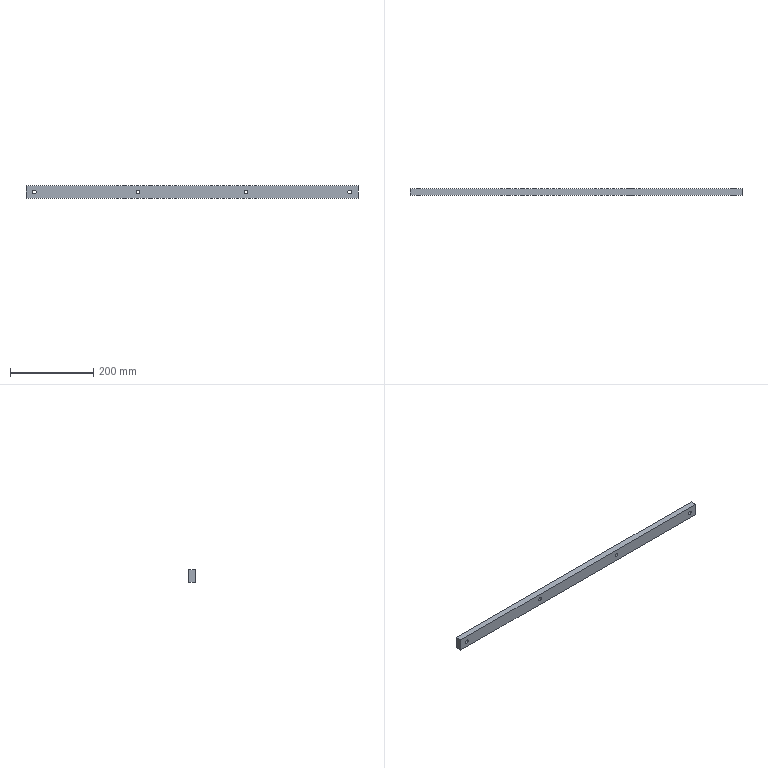Part | STEP file | 0244_210_Plate | 1 solid | 14 faces | box 800 x 15 x 30 mm | volume 356183 mm3 | cylinder 8 | plane 6 | commonest cylinder face diameters 9 x8
STEP:
#1=CARTESIAN_POINT('',(0.,0.,0.));
#2=DIRECTION('',(0.,0.,1.));
#3=DIRECTION('',(1.,0.,0.));
#4=AXIS2_PLACEMENT_3D('',#1,#2,#3);
#5=CARTESIAN_POINT('',(-130.,0.,19.5));
#6=VERTEX_POINT('',#5);
#7=CARTESIAN_POINT('',(-130.,15.,19.5));
#8=VERTEX_POINT('',#7);
#9=CARTESIAN_POINT('',(-130.,15.,19.5));
#10=DIRECTION('',(0.,1.,0.));
#11=VECTOR('',#10,1.);
#12=LINE('',#9,#11);
#13=CARTESIAN_POINT('',(-130.,15.,15.));
#14=DIRECTION('',(0.,1.,0.));
#15=DIRECTION('',(0.,0.,1.));
#16=AXIS2_PLACEMENT_3D('',#13,#14,#15);
#17=CYLINDRICAL_SURFACE('',#16,4.5);
#18=CARTESIAN_POINT('',(6.283,0.));
#19=DIRECTION('',(0.,1.));
#20=VECTOR('',#19,1.);
#21=LINE('',#18,#20);
#22=(GEOMETRIC_REPRESENTATION_CONTEXT(2)PARAMETRIC_REPRESENTATION_CONTEXT()REPRESENTATION_CONTEXT('',''));
#23=DEFINITIONAL_REPRESENTATION('',(#21),#22);
#24=PCURVE('',#17,#23);
#25=CARTESIAN_POINT('',(-130.,15.,15.));
#26=DIRECTION('',(0.,1.,0.));
#27=DIRECTION('',(0.,0.,1.));
#28=AXIS2_PLACEMENT_3D('',#25,#26,#27);
#29=CYLINDRICAL_SURFACE('',#28,4.5);
#30=CARTESIAN_POINT('',(0.,0.));
#31=DIRECTION('',(0.,1.));
#32=VECTOR('',#31,1.);
#33=LINE('',#30,#32);
#34=(GEOMETRIC_REPRESENTATION_CONTEXT(2)PARAMETRIC_REPRESENTATION_CONTEXT()REPRESENTATION_CONTEXT('',''));
#35=DEFINITIONAL_REPRESENTATION('',(#33),#34);
#36=PCURVE('',#29,#35);
#37=SURFACE_CURVE('',#12,(#24,#36),.PCURVE_S1.);
#38=EDGE_CURVE('',#6,#8,#37,.T.);
#39=ORIENTED_EDGE('',*,*,#38,.T.);
#40=CARTESIAN_POINT('',(-130.,15.,10.5));
#41=VERTEX_POINT('',#40);
#42=CARTESIAN_POINT('',(-130.,15.,15.));
#43=DIRECTION('',(0.,1.,0.));
#44=DIRECTION('',(0.,0.,1.));
#45=AXIS2_PLACEMENT_3D('',#42,#43,#44);
#46=CIRCLE('',#45,4.5);
#47=CARTESIAN_POINT('',(0.,0.));
#48=DIRECTION('',(1.,0.));
#49=VECTOR('',#48,1.);
#50=LINE('',#47,#49);
#51=(GEOMETRIC_REPRESENTATION_CONTEXT(2)PARAMETRIC_REPRESENTATION_CONTEXT()REPRESENTATION_CONTEXT('',''));
#52=DEFINITIONAL_REPRESENTATION('',(#50),#51);
#53=PCURVE('',#17,#52);
#54=CARTESIAN_POINT('',(-400.,15.,0.));
#55=DIRECTION('',(0.,1.,0.));
#56=DIRECTION('',(0.,0.,1.));
#57=AXIS2_PLACEMENT_3D('',#54,#55,#56);
#58=PLANE('',#57);
#59=CARTESIAN_POINT('',(15.,270.));
#60=DIRECTION('',(1.,0.));
#61=AXIS2_PLACEMENT_2D('',#59,#60);
#62=CIRCLE('',#61,4.5);
#63=(GEOMETRIC_REPRESENTATION_CONTEXT(2)PARAMETRIC_REPRESENTATION_CONTEXT()REPRESENTATION_CONTEXT('',''));
#64=DEFINITIONAL_REPRESENTATION('',(#62),#63);
#65=PCURVE('',#58,#64);
#66=SURFACE_CURVE('',#46,(#53,#65),.PCURVE_S1.);
#67=EDGE_CURVE('',#41,#8,#66,.T.);
#68=ORIENTED_EDGE('',*,*,#67,.F.);
#69=CARTESIAN_POINT('',(-130.,0.,10.5));
#70=VERTEX_POINT('',#69);
#71=CARTESIAN_POINT('',(-130.,15.,10.5));
#72=DIRECTION('',(0.,1.,0.));
#73=VECTOR('',#72,1.);
#74=LINE('',#71,#73);
#75=CARTESIAN_POINT('',(3.142,0.));
#76=DIRECTION('',(0.,1.));
#77=VECTOR('',#76,1.);
#78=LINE('',#75,#77);
#79=(GEOMETRIC_REPRESENTATION_CONTEXT(2)PARAMETRIC_REPRESENTATION_CONTEXT()REPRESENTATION_CONTEXT('',''));
#80=DEFINITIONAL_REPRESENTATION('',(#78),#79);
#81=PCURVE('',#17,#80);
#82=CARTESIAN_POINT('',(3.142,0.));
#83=DIRECTION('',(0.,1.));
#84=VECTOR('',#83,1.);
#85=LINE('',#82,#84);
#86=(GEOMETRIC_REPRESENTATION_CONTEXT(2)PARAMETRIC_REPRESENTATION_CONTEXT()REPRESENTATION_CONTEXT('',''));
#87=DEFINITIONAL_REPRESENTATION('',(#85),#86);
#88=PCURVE('',#29,#87);
#89=SURFACE_CURVE('',#74,(#81,#88),.PCURVE_S1.);
#90=EDGE_CURVE('',#70,#41,#89,.T.);
#91=ORIENTED_EDGE('',*,*,#90,.F.);
#92=CARTESIAN_POINT('',(-130.,0.,15.));
#93=DIRECTION('',(0.,1.,0.));
#94=DIRECTION('',(0.,0.,1.));
#95=AXIS2_PLACEMENT_3D('',#92,#93,#94);
#96=CIRCLE('',#95,4.5);
#97=CARTESIAN_POINT('',(0.,-15.));
#98=DIRECTION('',(1.,0.));
#99=VECTOR('',#98,1.);
#100=LINE('',#97,#99);
#101=(GEOMETRIC_REPRESENTATION_CONTEXT(2)PARAMETRIC_REPRESENTATION_CONTEXT()REPRESENTATION_CONTEXT('',''));
#102=DEFINITIONAL_REPRESENTATION('',(#100),#101);
#103=PCURVE('',#17,#102);
#104=CARTESIAN_POINT('',(-400.,0.,0.));
#105=DIRECTION('',(0.,1.,0.));
#106=DIRECTION('',(0.,0.,1.));
#107=AXIS2_PLACEMENT_3D('',#104,#105,#106);
#108=PLANE('',#107);
#109=CARTESIAN_POINT('',(15.,270.));
#110=DIRECTION('',(1.,0.));
#111=AXIS2_PLACEMENT_2D('',#109,#110);
#112=CIRCLE('',#111,4.5);
#113=(GEOMETRIC_REPRESENTATION_CONTEXT(2)PARAMETRIC_REPRESENTATION_CONTEXT()REPRESENTATION_CONTEXT('',''));
#114=DEFINITIONAL_REPRESENTATION('',(#112),#113);
#115=PCURVE('',#108,#114);
#116=SURFACE_CURVE('',#96,(#103,#115),.PCURVE_S1.);
#117=EDGE_CURVE('',#70,#6,#116,.T.);
#118=ORIENTED_EDGE('',*,*,#117,.T.);
#119=EDGE_LOOP('',(#39,#68,#91,#118));
#120=FACE_BOUND('',#119,.F.);
#121=ADVANCED_FACE('',(#120),#17,.F.);
#122=CARTESIAN_POINT('',(130.,0.,19.5));
#123=VERTEX_POINT('',#122);
#124=CARTESIAN_POINT('',(130.,15.,19.5));
#125=VERTEX_POINT('',#124);
#126=CARTESIAN_POINT('',(130.,15.,19.5));
#127=DIRECTION('',(0.,1.,0.));
#128=VECTOR('',#127,1.);
#129=LINE('',#126,#128);
#130=CARTESIAN_POINT('',(130.,15.,15.));
#131=DIRECTION('',(0.,1.,0.));
#132=DIRECTION('',(0.,0.,1.));
#133=AXIS2_PLACEMENT_3D('',#130,#131,#132);
#134=CYLINDRICAL_SURFACE('',#133,4.5);
#135=CARTESIAN_POINT('',(6.283,0.));
#136=DIRECTION('',(0.,1.));
#137=VECTOR('',#136,1.);
#138=LINE('',#135,#137);
#139=(GEOMETRIC_REPRESENTATION_CONTEXT(2)PARAMETRIC_REPRESENTATION_CONTEXT()REPRESENTATION_CONTEXT('',''));
#140=DEFINITIONAL_REPRESENTATION('',(#138),#139);
#141=PCURVE('',#134,#140);
#142=CARTESIAN_POINT('',(130.,15.,15.));
#143=DIRECTION('',(0.,1.,0.));
#144=DIRECTION('',(0.,0.,1.));
#145=AXIS2_PLACEMENT_3D('',#142,#143,#144);
#146=CYLINDRICAL_SURFACE('',#145,4.5);
#147=CARTESIAN_POINT('',(0.,0.));
#148=DIRECTION('',(0.,1.));
#149=VECTOR('',#148,1.);
#150=LINE('',#147,#149);
#151=(GEOMETRIC_REPRESENTATION_CONTEXT(2)PARAMETRIC_REPRESENTATION_CONTEXT()REPRESENTATION_CONTEXT('',''));
#152=DEFINITIONAL_REPRESENTATION('',(#150),#151);
#153=PCURVE('',#146,#152);
#154=SURFACE_CURVE('',#129,(#141,#153),.PCURVE_S1.);
#155=EDGE_CURVE('',#123,#125,#154,.T.);
#156=ORIENTED_EDGE('',*,*,#155,.T.);
#157=CARTESIAN_POINT('',(130.,15.,10.5));
#158=VERTEX_POINT('',#157);
#159=CARTESIAN_POINT('',(130.,15.,15.));
#160=DIRECTION('',(0.,1.,0.));
#161=DIRECTION('',(0.,0.,1.));
#162=AXIS2_PLACEMENT_3D('',#159,#160,#161);
#163=CIRCLE('',#162,4.5);
#164=CARTESIAN_POINT('',(0.,0.));
#165=DIRECTION('',(1.,0.));
#166=VECTOR('',#165,1.);
#167=LINE('',#164,#166);
#168=(GEOMETRIC_REPRESENTATION_CONTEXT(2)PARAMETRIC_REPRESENTATION_CONTEXT()REPRESENTATION_CONTEXT('',''));
#169=DEFINITIONAL_REPRESENTATION('',(#167),#168);
#170=PCURVE('',#134,#169);
#171=CARTESIAN_POINT('',(15.,530.));
#172=DIRECTION('',(1.,0.));
#173=AXIS2_PLACEMENT_2D('',#171,#172);
#174=CIRCLE('',#173,4.5);
#175=(GEOMETRIC_REPRESENTATION_CONTEXT(2)PARAMETRIC_REPRESENTATION_CONTEXT()REPRESENTATION_CONTEXT('',''));
#176=DEFINITIONAL_REPRESENTATION('',(#174),#175);
#177=PCURVE('',#58,#176);
#178=SURFACE_CURVE('',#163,(#170,#177),.PCURVE_S1.);
#179=EDGE_CURVE('',#158,#125,#178,.T.);
#180=ORIENTED_EDGE('',*,*,#179,.F.);
#181=CARTESIAN_POINT('',(130.,0.,10.5));
#182=VERTEX_POINT('',#181);
#183=CARTESIAN_POINT('',(130.,15.,10.5));
#184=DIRECTION('',(0.,1.,0.));
#185=VECTOR('',#184,1.);
#186=LINE('',#183,#185);
#187=CARTESIAN_POINT('',(3.142,0.));
#188=DIRECTION('',(0.,1.));
#189=VECTOR('',#188,1.);
#190=LINE('',#187,#189);
#191=(GEOMETRIC_REPRESENTATION_CONTEXT(2)PARAMETRIC_REPRESENTATION_CONTEXT()REPRESENTATION_CONTEXT('',''));
#192=DEFINITIONAL_REPRESENTATION('',(#190),#191);
#193=PCURVE('',#134,#192);
#194=CARTESIAN_POINT('',(3.142,0.));
#195=DIRECTION('',(0.,1.));
#196=VECTOR('',#195,1.);
#197=LINE('',#194,#196);
#198=(GEOMETRIC_REPRESENTATION_CONTEXT(2)PARAMETRIC_REPRESENTATION_CONTEXT()REPRESENTATION_CONTEXT('',''));
#199=DEFINITIONAL_REPRESENTATION('',(#197),#198);
#200=PCURVE('',#146,#199);
#201=SURFACE_CURVE('',#186,(#193,#200),.PCURVE_S1.);
#202=EDGE_CURVE('',#182,#158,#201,.T.);
#203=ORIENTED_EDGE('',*,*,#202,.F.);
#204=CARTESIAN_POINT('',(130.,0.,15.));
#205=DIRECTION('',(0.,1.,0.));
#206=DIRECTION('',(0.,0.,1.));
#207=AXIS2_PLACEMENT_3D('',#204,#205,#206);
#208=CIRCLE('',#207,4.5);
#209=CARTESIAN_POINT('',(0.,-15.));
#210=DIRECTION('',(1.,0.));
#211=VECTOR('',#210,1.);
#212=LINE('',#209,#211);
#213=(GEOMETRIC_REPRESENTATION_CONTEXT(2)PARAMETRIC_REPRESENTATION_CONTEXT()REPRESENTATION_CONTEXT('',''));
#214=DEFINITIONAL_REPRESENTATION('',(#212),#213);
#215=PCURVE('',#134,#214);
#216=CARTESIAN_POINT('',(15.,530.));
#217=DIRECTION('',(1.,0.));
#218=AXIS2_PLACEMENT_2D('',#216,#217);
#219=CIRCLE('',#218,4.5);
#220=(GEOMETRIC_REPRESENTATION_CONTEXT(2)PARAMETRIC_REPRESENTATION_CONTEXT()REPRESENTATION_CONTEXT('',''));
#221=DEFINITIONAL_REPRESENTATION('',(#219),#220);
#222=PCURVE('',#108,#221);
#223=SURFACE_CURVE('',#208,(#215,#222),.PCURVE_S1.);
#224=EDGE_CURVE('',#182,#123,#223,.T.);
#225=ORIENTED_EDGE('',*,*,#224,.T.);
#226=EDGE_LOOP('',(#156,#180,#203,#225));
#227=FACE_BOUND('',#226,.F.);
#228=ADVANCED_FACE('',(#227),#134,.F.);
#229=CARTESIAN_POINT('',(380.,0.,19.5));
#230=VERTEX_POINT('',#229);
#231=CARTESIAN_POINT('',(380.,15.,19.5));
#232=VERTEX_POINT('',#231);
#233=CARTESIAN_POINT('',(380.,15.,19.5));
#234=DIRECTION('',(0.,1.,0.));
#235=VECTOR('',#234,1.);
#236=LINE('',#233,#235);
#237=CARTESIAN_POINT('',(380.,15.,15.));
#238=DIRECTION('',(0.,1.,0.));
#239=DIRECTION('',(0.,0.,1.));
#240=AXIS2_PLACEMENT_3D('',#237,#238,#239);
#241=CYLINDRICAL_SURFACE('',#240,4.5);
#242=CARTESIAN_POINT('',(6.283,0.));
#243=DIRECTION('',(0.,1.));
#244=VECTOR('',#243,1.);
#245=LINE('',#242,#244);
#246=(GEOMETRIC_REPRESENTATION_CONTEXT(2)PARAMETRIC_REPRESENTATION_CONTEXT()REPRESENTATION_CONTEXT('',''));
#247=DEFINITIONAL_REPRESENTATION('',(#245),#246);
#248=PCURVE('',#241,#247);
#249=CARTESIAN_POINT('',(380.,15.,15.));
#250=DIRECTION('',(0.,1.,0.));
#251=DIRECTION('',(0.,0.,1.));
#252=AXIS2_PLACEMENT_3D('',#249,#250,#251);
#253=CYLINDRICAL_SURFACE('',#252,4.5);
#254=CARTESIAN_POINT('',(0.,0.));
#255=DIRECTION('',(0.,1.));
#256=VECTOR('',#255,1.);
#257=LINE('',#254,#256);
#258=(GEOMETRIC_REPRESENTATION_CONTEXT(2)PARAMETRIC_REPRESENTATION_CONTEXT()REPRESENTATION_CONTEXT('',''));
#259=DEFINITIONAL_REPRESENTATION('',(#257),#258);
#260=PCURVE('',#253,#259);
#261=SURFACE_CURVE('',#236,(#248,#260),.PCURVE_S1.);
#262=EDGE_CURVE('',#230,#232,#261,.T.);
#263=ORIENTED_EDGE('',*,*,#262,.T.);
#264=CARTESIAN_POINT('',(380.,15.,10.5));
#265=VERTEX_POINT('',#264);
#266=CARTESIAN_POINT('',(380.,15.,15.));
#267=DIRECTION('',(0.,1.,0.));
#268=DIRECTION('',(0.,0.,1.));
#269=AXIS2_PLACEMENT_3D('',#266,#267,#268);
#270=CIRCLE('',#269,4.5);
#271=CARTESIAN_POINT('',(0.,0.));
#272=DIRECTION('',(1.,0.));
#273=VECTOR('',#272,1.);
#274=LINE('',#271,#273);
#275=(GEOMETRIC_REPRESENTATION_CONTEXT(2)PARAMETRIC_REPRESENTATION_CONTEXT()REPRESENTATION_CONTEXT('',''));
#276=DEFINITIONAL_REPRESENTATION('',(#274),#275);
#277=PCURVE('',#241,#276);
#278=CARTESIAN_POINT('',(15.,780.));
#279=DIRECTION('',(1.,0.));
#280=AXIS2_PLACEMENT_2D('',#278,#279);
#281=CIRCLE('',#280,4.5);
#282=(GEOMETRIC_REPRESENTATION_CONTEXT(2)PARAMETRIC_REPRESENTATION_CONTEXT()REPRESENTATION_CONTEXT('',''));
#283=DEFINITIONAL_REPRESENTATION('',(#281),#282);
#284=PCURVE('',#58,#283);
#285=SURFACE_CURVE('',#270,(#277,#284),.PCURVE_S1.);
#286=EDGE_CURVE('',#265,#232,#285,.T.);
#287=ORIENTED_EDGE('',*,*,#286,.F.);
#288=CARTESIAN_POINT('',(380.,0.,10.5));
#289=VERTEX_POINT('',#288);
#290=CARTESIAN_POINT('',(380.,15.,10.5));
#291=DIRECTION('',(0.,1.,0.));
#292=VECTOR('',#291,1.);
#293=LINE('',#290,#292);
#294=CARTESIAN_POINT('',(3.142,0.));
#295=DIRECTION('',(0.,1.));
#296=VECTOR('',#295,1.);
#297=LINE('',#294,#296);
#298=(GEOMETRIC_REPRESENTATION_CONTEXT(2)PARAMETRIC_REPRESENTATION_CONTEXT()REPRESENTATION_CONTEXT('',''));
#299=DEFINITIONAL_REPRESENTATION('',(#297),#298);
#300=PCURVE('',#241,#299);
#301=CARTESIAN_POINT('',(3.142,0.));
#302=DIRECTION('',(0.,1.));
#303=VECTOR('',#302,1.);
#304=LINE('',#301,#303);
#305=(GEOMETRIC_REPRESENTATION_CONTEXT(2)PARAMETRIC_REPRESENTATION_CONTEXT()REPRESENTATION_CONTEXT('',''));
#306=DEFINITIONAL_REPRESENTATION('',(#304),#305);
#307=PCURVE('',#253,#306);
#308=SURFACE_CURVE('',#293,(#300,#307),.PCURVE_S1.);
#309=EDGE_CURVE('',#289,#265,#308,.T.);
#310=ORIENTED_EDGE('',*,*,#309,.F.);
#311=CARTESIAN_POINT('',(380.,0.,15.));
#312=DIRECTION('',(0.,1.,0.));
#313=DIRECTION('',(0.,0.,1.));
#314=AXIS2_PLACEMENT_3D('',#311,#312,#313);
#315=CIRCLE('',#314,4.5);
#316=CARTESIAN_POINT('',(0.,-15.));
#317=DIRECTION('',(1.,0.));
#318=VECTOR('',#317,1.);
#319=LINE('',#316,#318);
#320=(GEOMETRIC_REPRESENTATION_CONTEXT(2)PARAMETRIC_REPRESENTATION_CONTEXT()REPRESENTATION_CONTEXT('',''));
#321=DEFINITIONAL_REPRESENTATION('',(#319),#320);
#322=PCURVE('',#241,#321);
#323=CARTESIAN_POINT('',(15.,780.));
#324=DIRECTION('',(1.,0.));
#325=AXIS2_PLACEMENT_2D('',#323,#324);
#326=CIRCLE('',#325,4.5);
#327=(GEOMETRIC_REPRESENTATION_CONTEXT(2)PARAMETRIC_REPRESENTATION_CONTEXT()REPRESENTATION_CONTEXT('',''));
#328=DEFINITIONAL_REPRESENTATION('',(#326),#327);
#329=PCURVE('',#108,#328);
#330=SURFACE_CURVE('',#315,(#322,#329),.PCURVE_S1.);
#331=EDGE_CURVE('',#289,#230,#330,.T.);
#332=ORIENTED_EDGE('',*,*,#331,.T.);
#333=EDGE_LOOP('',(#263,#287,#310,#332));
#334=FACE_BOUND('',#333,.F.);
#335=ADVANCED_FACE('',(#334),#241,.F.);
#336=CARTESIAN_POINT('',(-380.,0.,19.5));
#337=VERTEX_POINT('',#336);
#338=CARTESIAN_POINT('',(-380.,15.,19.5));
#339=VERTEX_POINT('',#338);
#340=CARTESIAN_POINT('',(-380.,15.,19.5));
#341=DIRECTION('',(0.,1.,0.));
#342=VECTOR('',#341,1.);
#343=LINE('',#340,#342);
#344=CARTESIAN_POINT('',(-380.,15.,15.));
#345=DIRECTION('',(0.,1.,0.));
#346=DIRECTION('',(0.,0.,1.));
#347=AXIS2_PLACEMENT_3D('',#344,#345,#346);
#348=CYLINDRICAL_SURFACE('',#347,4.5);
#349=CARTESIAN_POINT('',(6.283,0.));
#350=DIRECTION('',(0.,1.));
#351=VECTOR('',#350,1.);
#352=LINE('',#349,#351);
#353=(GEOMETRIC_REPRESENTATION_CONTEXT(2)PARAMETRIC_REPRESENTATION_CONTEXT()REPRESENTATION_CONTEXT('',''));
#354=DEFINITIONAL_REPRESENTATION('',(#352),#353);
#355=PCURVE('',#348,#354);
#356=CARTESIAN_POINT('',(-380.,15.,15.));
#357=DIRECTION('',(0.,1.,0.));
#358=DIRECTION('',(0.,0.,1.));
#359=AXIS2_PLACEMENT_3D('',#356,#357,#358);
#360=CYLINDRICAL_SURFACE('',#359,4.5);
#361=CARTESIAN_POINT('',(0.,0.));
#362=DIRECTION('',(0.,1.));
#363=VECTOR('',#362,1.);
#364=LINE('',#361,#363);
#365=(GEOMETRIC_REPRESENTATION_CONTEXT(2)PARAMETRIC_REPRESENTATION_CONTEXT()REPRESENTATION_CONTEXT('',''));
#366=DEFINITIONAL_REPRESENTATION('',(#364),#365);
#367=PCURVE('',#360,#366);
#368=SURFACE_CURVE('',#343,(#355,#367),.PCURVE_S1.);
#369=EDGE_CURVE('',#337,#339,#368,.T.);
#370=ORIENTED_EDGE('',*,*,#369,.T.);
#371=CARTESIAN_POINT('',(-380.,15.,10.5));
#372=VERTEX_POINT('',#371);
#373=CARTESIAN_POINT('',(-380.,15.,15.));
#374=DIRECTION('',(0.,1.,0.));
#375=DIRECTION('',(0.,0.,1.));
#376=AXIS2_PLACEMENT_3D('',#373,#374,#375);
#377=CIRCLE('',#376,4.5);
#378=CARTESIAN_POINT('',(0.,0.));
#379=DIRECTION('',(1.,0.));
#380=VECTOR('',#379,1.);
#381=LINE('',#378,#380);
#382=(GEOMETRIC_REPRESENTATION_CONTEXT(2)PARAMETRIC_REPRESENTATION_CONTEXT()REPRESENTATION_CONTEXT('',''));
#383=DEFINITIONAL_REPRESENTATION('',(#381),#382);
#384=PCURVE('',#348,#383);
#385=CARTESIAN_POINT('',(15.,20.));
#386=DIRECTION('',(1.,0.));
#387=AXIS2_PLACEMENT_2D('',#385,#386);
#388=CIRCLE('',#387,4.5);
#389=(GEOMETRIC_REPRESENTATION_CONTEXT(2)PARAMETRIC_REPRESENTATION_CONTEXT()REPRESENTATION_CONTEXT('',''));
#390=DEFINITIONAL_REPRESENTATION('',(#388),#389);
#391=PCURVE('',#58,#390);
#392=SURFACE_CURVE('',#377,(#384,#391),.PCURVE_S1.);
#393=EDGE_CURVE('',#372,#339,#392,.T.);
#394=ORIENTED_EDGE('',*,*,#393,.F.);
#395=CARTESIAN_POINT('',(-380.,0.,10.5));
#396=VERTEX_POINT('',#395);
#397=CARTESIAN_POINT('',(-380.,15.,10.5));
#398=DIRECTION('',(0.,1.,0.));
#399=VECTOR('',#398,1.);
#400=LINE('',#397,#399);
#401=CARTESIAN_POINT('',(3.142,0.));
#402=DIRECTION('',(0.,1.));
#403=VECTOR('',#402,1.);
#404=LINE('',#401,#403);
#405=(GEOMETRIC_REPRESENTATION_CONTEXT(2)PARAMETRIC_REPRESENTATION_CONTEXT()REPRESENTATION_CONTEXT('',''));
#406=DEFINITIONAL_REPRESENTATION('',(#404),#405);
#407=PCURVE('',#348,#406);
#408=CARTESIAN_POINT('',(3.142,0.));
#409=DIRECTION('',(0.,1.));
#410=VECTOR('',#409,1.);
#411=LINE('',#408,#410);
#412=(GEOMETRIC_REPRESENTATION_CONTEXT(2)PARAMETRIC_REPRESENTATION_CONTEXT()REPRESENTATION_CONTEXT('',''));
#413=DEFINITIONAL_REPRESENTATION('',(#411),#412);
#414=PCURVE('',#360,#413);
#415=SURFACE_CURVE('',#400,(#407,#414),.PCURVE_S1.);
#416=EDGE_CURVE('',#396,#372,#415,.T.);
#417=ORIENTED_EDGE('',*,*,#416,.F.);
#418=CARTESIAN_POINT('',(-380.,0.,15.));
#419=DIRECTION('',(0.,1.,0.));
#420=DIRECTION('',(0.,0.,1.));
#421=AXIS2_PLACEMENT_3D('',#418,#419,#420);
#422=CIRCLE('',#421,4.5);
#423=CARTESIAN_POINT('',(0.,-15.));
#424=DIRECTION('',(1.,0.));
#425=VECTOR('',#424,1.);
#426=LINE('',#423,#425);
#427=(GEOMETRIC_REPRESENTATION_CONTEXT(2)PARAMETRIC_REPRESENTATION_CONTEXT()REPRESENTATION_CONTEXT('',''));
#428=DEFINITIONAL_REPRESENTATION('',(#426),#427);
#429=PCURVE('',#348,#428);
#430=CARTESIAN_POINT('',(15.,20.));
#431=DIRECTION('',(1.,0.));
#432=AXIS2_PLACEMENT_2D('',#430,#431);
#433=CIRCLE('',#432,4.5);
#434=(GEOMETRIC_REPRESENTATION_CONTEXT(2)PARAMETRIC_REPRESENTATION_CONTEXT()REPRESENTATION_CONTEXT('',''));
#435=DEFINITIONAL_REPRESENTATION('',(#433),#434);
#436=PCURVE('',#108,#435);
#437=SURFACE_CURVE('',#422,(#429,#436),.PCURVE_S1.);
#438=EDGE_CURVE('',#396,#337,#437,.T.);
#439=ORIENTED_EDGE('',*,*,#438,.T.);
#440=EDGE_LOOP('',(#370,#394,#417,#439));
#441=FACE_BOUND('',#440,.F.);
#442=ADVANCED_FACE('',(#441),#348,.F.);
#443=CARTESIAN_POINT('',(400.,0.,0.));
#444=VERTEX_POINT('',#443);
#445=CARTESIAN_POINT('',(-400.,0.,0.));
#446=VERTEX_POINT('',#445);
#447=CARTESIAN_POINT('',(400.,0.,0.));
#448=DIRECTION('',(-1.,0.,0.));
#449=VECTOR('',#448,1.);
#450=LINE('',#447,#449);
#451=CARTESIAN_POINT('',(400.,15.,0.));
#452=DIRECTION('',(0.,0.,1.));
#453=DIRECTION('',(1.,0.,0.));
#454=AXIS2_PLACEMENT_3D('',#451,#452,#453);
#455=PLANE('',#454);
#456=CARTESIAN_POINT('',(0.,-15.));
#457=DIRECTION('',(-1.,0.));
#458=VECTOR('',#457,1.);
#459=LINE('',#456,#458);
#460=(GEOMETRIC_REPRESENTATION_CONTEXT(2)PARAMETRIC_REPRESENTATION_CONTEXT()REPRESENTATION_CONTEXT('',''));
#461=DEFINITIONAL_REPRESENTATION('',(#459),#460);
#462=PCURVE('',#455,#461);
#463=CARTESIAN_POINT('',(0.,800.));
#464=DIRECTION('',(0.,-1.));
#465=VECTOR('',#464,1.);
#466=LINE('',#463,#465);
#467=(GEOMETRIC_REPRESENTATION_CONTEXT(2)PARAMETRIC_REPRESENTATION_CONTEXT()REPRESENTATION_CONTEXT('',''));
#468=DEFINITIONAL_REPRESENTATION('',(#466),#467);
#469=PCURVE('',#108,#468);
#470=SURFACE_CURVE('',#450,(#462,#469),.PCURVE_S1.);
#471=EDGE_CURVE('',#444,#446,#470,.T.);
#472=ORIENTED_EDGE('',*,*,#471,.T.);
#473=CARTESIAN_POINT('',(-400.,15.,0.));
#474=VERTEX_POINT('',#473);
#475=CARTESIAN_POINT('',(-400.,15.,0.));
#476=DIRECTION('',(0.,-1.,0.));
#477=VECTOR('',#476,1.);
#478=LINE('',#475,#477);
#479=CARTESIAN_POINT('',(-800.,0.));
#480=DIRECTION('',(0.,-1.));
#481=VECTOR('',#480,1.);
#482=LINE('',#479,#481);
#483=(GEOMETRIC_REPRESENTATION_CONTEXT(2)PARAMETRIC_REPRESENTATION_CONTEXT()REPRESENTATION_CONTEXT('',''));
#484=DEFINITIONAL_REPRESENTATION('',(#482),#483);
#485=PCURVE('',#455,#484);
#486=CARTESIAN_POINT('',(-400.,15.,0.));
#487=DIRECTION('',(1.,0.,0.));
#488=DIRECTION('',(0.,0.,-1.));
#489=AXIS2_PLACEMENT_3D('',#486,#487,#488);
#490=PLANE('',#489);
#491=CARTESIAN_POINT('',(0.,0.));
#492=DIRECTION('',(0.,-1.));
#493=VECTOR('',#492,1.);
#494=LINE('',#491,#493);
#495=(GEOMETRIC_REPRESENTATION_CONTEXT(2)PARAMETRIC_REPRESENTATION_CONTEXT()REPRESENTATION_CONTEXT('',''));
#496=DEFINITIONAL_REPRESENTATION('',(#494),#495);
#497=PCURVE('',#490,#496);
#498=SURFACE_CURVE('',#478,(#485,#497),.PCURVE_S1.);
#499=EDGE_CURVE('',#474,#446,#498,.T.);
#500=ORIENTED_EDGE('',*,*,#499,.F.);
#501=CARTESIAN_POINT('',(400.,15.,0.));
#502=VERTEX_POINT('',#501);
#503=CARTESIAN_POINT('',(400.,15.,0.));
#504=DIRECTION('',(-1.,0.,0.));
#505=VECTOR('',#504,1.);
#506=LINE('',#503,#505);
#507=CARTESIAN_POINT('',(0.,0.));
#508=DIRECTION('',(-1.,0.));
#509=VECTOR('',#508,1.);
#510=LINE('',#507,#509);
#511=(GEOMETRIC_REPRESENTATION_CONTEXT(2)PARAMETRIC_REPRESENTATION_CONTEXT()REPRESENTATION_CONTEXT('',''));
#512=DEFINITIONAL_REPRESENTATION('',(#510),#511);
#513=PCURVE('',#455,#512);
#514=CARTESIAN_POINT('',(0.,800.));
#515=DIRECTION('',(0.,-1.));
#516=VECTOR('',#515,1.);
#517=LINE('',#514,#516);
#518=(GEOMETRIC_REPRESENTATION_CONTEXT(2)PARAMETRIC_REPRESENTATION_CONTEXT()REPRESENTATION_CONTEXT('',''));
#519=DEFINITIONAL_REPRESENTATION('',(#517),#518);
#520=PCURVE('',#58,#519);
#521=SURFACE_CURVE('',#506,(#513,#520),.PCURVE_S1.);
#522=EDGE_CURVE('',#502,#474,#521,.T.);
#523=ORIENTED_EDGE('',*,*,#522,.F.);
#524=CARTESIAN_POINT('',(400.,15.,0.));
#525=DIRECTION('',(0.,-1.,0.));
#526=VECTOR('',#525,1.);
#527=LINE('',#524,#526);
#528=CARTESIAN_POINT('',(0.,0.));
#529=DIRECTION('',(0.,-1.));
#530=VECTOR('',#529,1.);
#531=LINE('',#528,#530);
#532=(GEOMETRIC_REPRESENTATION_CONTEXT(2)PARAMETRIC_REPRESENTATION_CONTEXT()REPRESENTATION_CONTEXT('',''));
#533=DEFINITIONAL_REPRESENTATION('',(#531),#532);
#534=PCURVE('',#455,#533);
#535=CARTESIAN_POINT('',(400.,15.,0.));
#536=DIRECTION('',(-1.,0.,0.));
#537=DIRECTION('',(0.,0.,1.));
#538=AXIS2_PLACEMENT_3D('',#535,#536,#537);
#539=PLANE('',#538);
#540=CARTESIAN_POINT('',(0.,0.));
#541=DIRECTION('',(0.,-1.));
#542=VECTOR('',#541,1.);
#543=LINE('',#540,#542);
#544=(GEOMETRIC_REPRESENTATION_CONTEXT(2)PARAMETRIC_REPRESENTATION_CONTEXT()REPRESENTATION_CONTEXT('',''));
#545=DEFINITIONAL_REPRESENTATION('',(#543),#544);
#546=PCURVE('',#539,#545);
#547=SURFACE_CURVE('',#527,(#534,#546),.PCURVE_S1.);
#548=EDGE_CURVE('',#502,#444,#547,.T.);
#549=ORIENTED_EDGE('',*,*,#548,.T.);
#550=EDGE_LOOP('',(#472,#500,#523,#549));
#551=FACE_BOUND('',#550,.T.);
#552=ADVANCED_FACE('',(#551),#455,.F.);
#553=CARTESIAN_POINT('',(-400.,0.,30.));
#554=VERTEX_POINT('',#553);
#555=CARTESIAN_POINT('',(-400.,0.,0.));
#556=DIRECTION('',(0.,0.,1.));
#557=VECTOR('',#556,1.);
#558=LINE('',#555,#557);
#559=CARTESIAN_POINT('',(0.,-15.));
#560=DIRECTION('',(-1.,0.));
#561=VECTOR('',#560,1.);
#562=LINE('',#559,#561);
#563=(GEOMETRIC_REPRESENTATION_CONTEXT(2)PARAMETRIC_REPRESENTATION_CONTEXT()REPRESENTATION_CONTEXT('',''));
#564=DEFINITIONAL_REPRESENTATION('',(#562),#563);
#565=PCURVE('',#490,#564);
#566=CARTESIAN_POINT('',(0.,0.));
#567=DIRECTION('',(1.,0.));
#568=VECTOR('',#567,1.);
#569=LINE('',#566,#568);
#570=(GEOMETRIC_REPRESENTATION_CONTEXT(2)PARAMETRIC_REPRESENTATION_CONTEXT()REPRESENTATION_CONTEXT('',''));
#571=DEFINITIONAL_REPRESENTATION('',(#569),#570);
#572=PCURVE('',#108,#571);
#573=SURFACE_CURVE('',#558,(#565,#572),.PCURVE_S1.);
#574=EDGE_CURVE('',#446,#554,#573,.T.);
#575=ORIENTED_EDGE('',*,*,#574,.T.);
#576=CARTESIAN_POINT('',(-400.,15.,30.));
#577=VERTEX_POINT('',#576);
#578=CARTESIAN_POINT('',(-400.,15.,30.));
#579=DIRECTION('',(0.,-1.,0.));
#580=VECTOR('',#579,1.);
#581=LINE('',#578,#580);
#582=CARTESIAN_POINT('',(-30.,0.));
#583=DIRECTION('',(0.,-1.));
#584=VECTOR('',#583,1.);
#585=LINE('',#582,#584);
#586=(GEOMETRIC_REPRESENTATION_CONTEXT(2)PARAMETRIC_REPRESENTATION_CONTEXT()REPRESENTATION_CONTEXT('',''));
#587=DEFINITIONAL_REPRESENTATION('',(#585),#586);
#588=PCURVE('',#490,#587);
#589=CARTESIAN_POINT('',(400.,15.,30.));
#590=DIRECTION('',(0.,0.,-1.));
#591=DIRECTION('',(-1.,0.,0.));
#592=AXIS2_PLACEMENT_3D('',#589,#590,#591);
#593=PLANE('',#592);
#594=CARTESIAN_POINT('',(800.,0.));
#595=DIRECTION('',(0.,-1.));
#596=VECTOR('',#595,1.);
#597=LINE('',#594,#596);
#598=(GEOMETRIC_REPRESENTATION_CONTEXT(2)PARAMETRIC_REPRESENTATION_CONTEXT()REPRESENTATION_CONTEXT('',''));
#599=DEFINITIONAL_REPRESENTATION('',(#597),#598);
#600=PCURVE('',#593,#599);
#601=SURFACE_CURVE('',#581,(#588,#600),.PCURVE_S1.);
#602=EDGE_CURVE('',#577,#554,#601,.T.);
#603=ORIENTED_EDGE('',*,*,#602,.F.);
#604=CARTESIAN_POINT('',(-400.,15.,0.));
#605=DIRECTION('',(0.,0.,1.));
#606=VECTOR('',#605,1.);
#607=LINE('',#604,#606);
#608=CARTESIAN_POINT('',(0.,0.));
#609=DIRECTION('',(-1.,0.));
#610=VECTOR('',#609,1.);
#611=LINE('',#608,#610);
#612=(GEOMETRIC_REPRESENTATION_CONTEXT(2)PARAMETRIC_REPRESENTATION_CONTEXT()REPRESENTATION_CONTEXT('',''));
#613=DEFINITIONAL_REPRESENTATION('',(#611),#612);
#614=PCURVE('',#490,#613);
#615=CARTESIAN_POINT('',(0.,0.));
#616=DIRECTION('',(1.,0.));
#617=VECTOR('',#616,1.);
#618=LINE('',#615,#617);
#619=(GEOMETRIC_REPRESENTATION_CONTEXT(2)PARAMETRIC_REPRESENTATION_CONTEXT()REPRESENTATION_CONTEXT('',''));
#620=DEFINITIONAL_REPRESENTATION('',(#618),#619);
#621=PCURVE('',#58,#620);
#622=SURFACE_CURVE('',#607,(#614,#621),.PCURVE_S1.);
#623=EDGE_CURVE('',#474,#577,#622,.T.);
#624=ORIENTED_EDGE('',*,*,#623,.F.);
#625=ORIENTED_EDGE('',*,*,#499,.T.);
#626=EDGE_LOOP('',(#575,#603,#624,#625));
#627=FACE_BOUND('',#626,.T.);
#628=ADVANCED_FACE('',(#627),#490,.F.);
#629=CARTESIAN_POINT('',(400.,0.,30.));
#630=VERTEX_POINT('',#629);
#631=CARTESIAN_POINT('',(400.,0.,30.));
#632=DIRECTION('',(1.,0.,0.));
#633=VECTOR('',#632,1.);
#634=LINE('',#631,#633);
#635=CARTESIAN_POINT('',(0.,-15.));
#636=DIRECTION('',(-1.,0.));
#637=VECTOR('',#636,1.);
#638=LINE('',#635,#637);
#639=(GEOMETRIC_REPRESENTATION_CONTEXT(2)PARAMETRIC_REPRESENTATION_CONTEXT()REPRESENTATION_CONTEXT('',''));
#640=DEFINITIONAL_REPRESENTATION('',(#638),#639);
#641=PCURVE('',#593,#640);
#642=CARTESIAN_POINT('',(30.,800.));
#643=DIRECTION('',(0.,1.));
#644=VECTOR('',#643,1.);
#645=LINE('',#642,#644);
#646=(GEOMETRIC_REPRESENTATION_CONTEXT(2)PARAMETRIC_REPRESENTATION_CONTEXT()REPRESENTATION_CONTEXT('',''));
#647=DEFINITIONAL_REPRESENTATION('',(#645),#646);
#648=PCURVE('',#108,#647);
#649=SURFACE_CURVE('',#634,(#641,#648),.PCURVE_S1.);
#650=EDGE_CURVE('',#554,#630,#649,.T.);
#651=ORIENTED_EDGE('',*,*,#650,.T.);
#652=CARTESIAN_POINT('',(400.,15.,30.));
#653=VERTEX_POINT('',#652);
#654=CARTESIAN_POINT('',(400.,15.,30.));
#655=DIRECTION('',(0.,-1.,0.));
#656=VECTOR('',#655,1.);
#657=LINE('',#654,#656);
#658=CARTESIAN_POINT('',(0.,0.));
#659=DIRECTION('',(0.,-1.));
#660=VECTOR('',#659,1.);
#661=LINE('',#658,#660);
#662=(GEOMETRIC_REPRESENTATION_CONTEXT(2)PARAMETRIC_REPRESENTATION_CONTEXT()REPRESENTATION_CONTEXT('',''));
#663=DEFINITIONAL_REPRESENTATION('',(#661),#662);
#664=PCURVE('',#593,#663);
#665=CARTESIAN_POINT('',(30.,0.));
#666=DIRECTION('',(0.,-1.));
#667=VECTOR('',#666,1.);
#668=LINE('',#665,#667);
#669=(GEOMETRIC_REPRESENTATION_CONTEXT(2)PARAMETRIC_REPRESENTATION_CONTEXT()REPRESENTATION_CONTEXT('',''));
#670=DEFINITIONAL_REPRESENTATION('',(#668),#669);
#671=PCURVE('',#539,#670);
#672=SURFACE_CURVE('',#657,(#664,#671),.PCURVE_S1.);
#673=EDGE_CURVE('',#653,#630,#672,.T.);
#674=ORIENTED_EDGE('',*,*,#673,.F.);
#675=CARTESIAN_POINT('',(400.,15.,30.));
#676=DIRECTION('',(1.,0.,0.));
#677=VECTOR('',#676,1.);
#678=LINE('',#675,#677);
#679=CARTESIAN_POINT('',(0.,0.));
#680=DIRECTION('',(-1.,0.));
#681=VECTOR('',#680,1.);
#682=LINE('',#679,#681);
#683=(GEOMETRIC_REPRESENTATION_CONTEXT(2)PARAMETRIC_REPRESENTATION_CONTEXT()REPRESENTATION_CONTEXT('',''));
#684=DEFINITIONAL_REPRESENTATION('',(#682),#683);
#685=PCURVE('',#593,#684);
#686=CARTESIAN_POINT('',(30.,800.));
#687=DIRECTION('',(0.,1.));
#688=VECTOR('',#687,1.);
#689=LINE('',#686,#688);
#690=(GEOMETRIC_REPRESENTATION_CONTEXT(2)PARAMETRIC_REPRESENTATION_CONTEXT()REPRESENTATION_CONTEXT('',''));
#691=DEFINITIONAL_REPRESENTATION('',(#689),#690);
#692=PCURVE('',#58,#691);
#693=SURFACE_CURVE('',#678,(#685,#692),.PCURVE_S1.);
#694=EDGE_CURVE('',#577,#653,#693,.T.);
#695=ORIENTED_EDGE('',*,*,#694,.F.);
#696=ORIENTED_EDGE('',*,*,#602,.T.);
#697=EDGE_LOOP('',(#651,#674,#695,#696));
#698=FACE_BOUND('',#697,.T.);
#699=ADVANCED_FACE('',(#698),#593,.F.);
#700=CARTESIAN_POINT('',(400.,0.,0.));
#701=DIRECTION('',(0.,0.,-1.));
#702=VECTOR('',#701,1.);
#703=LINE('',#700,#702);
#704=CARTESIAN_POINT('',(0.,-15.));
#705=DIRECTION('',(-1.,0.));
#706=VECTOR('',#705,1.);
#707=LINE('',#704,#706);
#708=(GEOMETRIC_REPRESENTATION_CONTEXT(2)PARAMETRIC_REPRESENTATION_CONTEXT()REPRESENTATION_CONTEXT('',''));
#709=DEFINITIONAL_REPRESENTATION('',(#707),#708);
#710=PCURVE('',#539,#709);
#711=CARTESIAN_POINT('',(0.,800.));
#712=DIRECTION('',(-1.,0.));
#713=VECTOR('',#712,1.);
#714=LINE('',#711,#713);
#715=(GEOMETRIC_REPRESENTATION_CONTEXT(2)PARAMETRIC_REPRESENTATION_CONTEXT()REPRESENTATION_CONTEXT('',''));
#716=DEFINITIONAL_REPRESENTATION('',(#714),#715);
#717=PCURVE('',#108,#716);
#718=SURFACE_CURVE('',#703,(#710,#717),.PCURVE_S1.);
#719=EDGE_CURVE('',#630,#444,#718,.T.);
#720=ORIENTED_EDGE('',*,*,#719,.T.);
#721=ORIENTED_EDGE('',*,*,#548,.F.);
#722=CARTESIAN_POINT('',(400.,15.,0.));
#723=DIRECTION('',(0.,0.,-1.));
#724=VECTOR('',#723,1.);
#725=LINE('',#722,#724);
#726=CARTESIAN_POINT('',(0.,0.));
#727=DIRECTION('',(-1.,0.));
#728=VECTOR('',#727,1.);
#729=LINE('',#726,#728);
#730=(GEOMETRIC_REPRESENTATION_CONTEXT(2)PARAMETRIC_REPRESENTATION_CONTEXT()REPRESENTATION_CONTEXT('',''));
#731=DEFINITIONAL_REPRESENTATION('',(#729),#730);
#732=PCURVE('',#539,#731);
#733=CARTESIAN_POINT('',(0.,800.));
#734=DIRECTION('',(-1.,0.));
#735=VECTOR('',#734,1.);
#736=LINE('',#733,#735);
#737=(GEOMETRIC_REPRESENTATION_CONTEXT(2)PARAMETRIC_REPRESENTATION_CONTEXT()REPRESENTATION_CONTEXT('',''));
#738=DEFINITIONAL_REPRESENTATION('',(#736),#737);
#739=PCURVE('',#58,#738);
#740=SURFACE_CURVE('',#725,(#732,#739),.PCURVE_S1.);
#741=EDGE_CURVE('',#653,#502,#740,.T.);
#742=ORIENTED_EDGE('',*,*,#741,.F.);
#743=ORIENTED_EDGE('',*,*,#673,.T.);
#744=EDGE_LOOP('',(#720,#721,#742,#743));
#745=FACE_BOUND('',#744,.T.);
#746=ADVANCED_FACE('',(#745),#539,.F.);
#747=CARTESIAN_POINT('',(-130.,15.,15.));
#748=DIRECTION('',(0.,1.,0.));
#749=DIRECTION('',(0.,0.,1.));
#750=AXIS2_PLACEMENT_3D('',#747,#748,#749);
#751=CIRCLE('',#750,4.5);
#752=CARTESIAN_POINT('',(15.,270.));
#753=DIRECTION('',(1.,0.));
#754=AXIS2_PLACEMENT_2D('',#752,#753);
#755=CIRCLE('',#754,4.5);
#756=(GEOMETRIC_REPRESENTATION_CONTEXT(2)PARAMETRIC_REPRESENTATION_CONTEXT()REPRESENTATION_CONTEXT('',''));
#757=DEFINITIONAL_REPRESENTATION('',(#755),#756);
#758=PCURVE('',#58,#757);
#759=CARTESIAN_POINT('',(0.,0.));
#760=DIRECTION('',(1.,0.));
#761=VECTOR('',#760,1.);
#762=LINE('',#759,#761);
#763=(GEOMETRIC_REPRESENTATION_CONTEXT(2)PARAMETRIC_REPRESENTATION_CONTEXT()REPRESENTATION_CONTEXT('',''));
#764=DEFINITIONAL_REPRESENTATION('',(#762),#763);
#765=PCURVE('',#29,#764);
#766=SURFACE_CURVE('',#751,(#758,#765),.PCURVE_S1.);
#767=EDGE_CURVE('',#8,#41,#766,.T.);
#768=ORIENTED_EDGE('',*,*,#767,.F.);
#769=ORIENTED_EDGE('',*,*,#67,.F.);
#770=EDGE_LOOP('',(#768,#769));
#771=FACE_BOUND('',#770,.T.);
#772=CARTESIAN_POINT('',(130.,15.,15.));
#773=DIRECTION('',(0.,1.,0.));
#774=DIRECTION('',(0.,0.,1.));
#775=AXIS2_PLACEMENT_3D('',#772,#773,#774);
#776=CIRCLE('',#775,4.5);
#777=CARTESIAN_POINT('',(15.,530.));
#778=DIRECTION('',(1.,0.));
#779=AXIS2_PLACEMENT_2D('',#777,#778);
#780=CIRCLE('',#779,4.5);
#781=(GEOMETRIC_REPRESENTATION_CONTEXT(2)PARAMETRIC_REPRESENTATION_CONTEXT()REPRESENTATION_CONTEXT('',''));
#782=DEFINITIONAL_REPRESENTATION('',(#780),#781);
#783=PCURVE('',#58,#782);
#784=CARTESIAN_POINT('',(0.,0.));
#785=DIRECTION('',(1.,0.));
#786=VECTOR('',#785,1.);
#787=LINE('',#784,#786);
#788=(GEOMETRIC_REPRESENTATION_CONTEXT(2)PARAMETRIC_REPRESENTATION_CONTEXT()REPRESENTATION_CONTEXT('',''));
#789=DEFINITIONAL_REPRESENTATION('',(#787),#788);
#790=PCURVE('',#146,#789);
#791=SURFACE_CURVE('',#776,(#783,#790),.PCURVE_S1.);
#792=EDGE_CURVE('',#125,#158,#791,.T.);
#793=ORIENTED_EDGE('',*,*,#792,.F.);
#794=ORIENTED_EDGE('',*,*,#179,.F.);
#795=EDGE_LOOP('',(#793,#794));
#796=FACE_BOUND('',#795,.T.);
#797=CARTESIAN_POINT('',(380.,15.,15.));
#798=DIRECTION('',(0.,1.,0.));
#799=DIRECTION('',(0.,0.,1.));
#800=AXIS2_PLACEMENT_3D('',#797,#798,#799);
#801=CIRCLE('',#800,4.5);
#802=CARTESIAN_POINT('',(15.,780.));
#803=DIRECTION('',(1.,0.));
#804=AXIS2_PLACEMENT_2D('',#802,#803);
#805=CIRCLE('',#804,4.5);
#806=(GEOMETRIC_REPRESENTATION_CONTEXT(2)PARAMETRIC_REPRESENTATION_CONTEXT()REPRESENTATION_CONTEXT('',''));
#807=DEFINITIONAL_REPRESENTATION('',(#805),#806);
#808=PCURVE('',#58,#807);
#809=CARTESIAN_POINT('',(0.,0.));
#810=DIRECTION('',(1.,0.));
#811=VECTOR('',#810,1.);
#812=LINE('',#809,#811);
#813=(GEOMETRIC_REPRESENTATION_CONTEXT(2)PARAMETRIC_REPRESENTATION_CONTEXT()REPRESENTATION_CONTEXT('',''));
#814=DEFINITIONAL_REPRESENTATION('',(#812),#813);
#815=PCURVE('',#253,#814);
#816=SURFACE_CURVE('',#801,(#808,#815),.PCURVE_S1.);
#817=EDGE_CURVE('',#232,#265,#816,.T.);
#818=ORIENTED_EDGE('',*,*,#817,.F.);
#819=ORIENTED_EDGE('',*,*,#286,.F.);
#820=EDGE_LOOP('',(#818,#819));
#821=FACE_BOUND('',#820,.T.);
#822=CARTESIAN_POINT('',(-380.,15.,15.));
#823=DIRECTION('',(0.,1.,0.));
#824=DIRECTION('',(0.,0.,1.));
#825=AXIS2_PLACEMENT_3D('',#822,#823,#824);
#826=CIRCLE('',#825,4.5);
#827=CARTESIAN_POINT('',(15.,20.));
#828=DIRECTION('',(1.,0.));
#829=AXIS2_PLACEMENT_2D('',#827,#828);
#830=CIRCLE('',#829,4.5);
#831=(GEOMETRIC_REPRESENTATION_CONTEXT(2)PARAMETRIC_REPRESENTATION_CONTEXT()REPRESENTATION_CONTEXT('',''));
#832=DEFINITIONAL_REPRESENTATION('',(#830),#831);
#833=PCURVE('',#58,#832);
#834=CARTESIAN_POINT('',(0.,0.));
#835=DIRECTION('',(1.,0.));
#836=VECTOR('',#835,1.);
#837=LINE('',#834,#836);
#838=(GEOMETRIC_REPRESENTATION_CONTEXT(2)PARAMETRIC_REPRESENTATION_CONTEXT()REPRESENTATION_CONTEXT('',''));
#839=DEFINITIONAL_REPRESENTATION('',(#837),#838);
#840=PCURVE('',#360,#839);
#841=SURFACE_CURVE('',#826,(#833,#840),.PCURVE_S1.);
#842=EDGE_CURVE('',#339,#372,#841,.T.);
#843=ORIENTED_EDGE('',*,*,#842,.F.);
#844=ORIENTED_EDGE('',*,*,#393,.F.);
#845=EDGE_LOOP('',(#843,#844));
#846=FACE_BOUND('',#845,.T.);
#847=ORIENTED_EDGE('',*,*,#522,.T.);
#848=ORIENTED_EDGE('',*,*,#623,.T.);
#849=ORIENTED_EDGE('',*,*,#694,.T.);
#850=ORIENTED_EDGE('',*,*,#741,.T.);
#851=EDGE_LOOP('',(#847,#848,#849,#850));
#852=FACE_BOUND('',#851,.T.);
#853=ADVANCED_FACE('',(#771,#796,#821,#846,#852),#58,.T.);
#854=CARTESIAN_POINT('',(-130.,0.,15.));
#855=DIRECTION('',(0.,1.,0.));
#856=DIRECTION('',(0.,0.,1.));
#857=AXIS2_PLACEMENT_3D('',#854,#855,#856);
#858=CIRCLE('',#857,4.5);
#859=CARTESIAN_POINT('',(15.,270.));
#860=DIRECTION('',(1.,0.));
#861=AXIS2_PLACEMENT_2D('',#859,#860);
#862=CIRCLE('',#861,4.5);
#863=(GEOMETRIC_REPRESENTATION_CONTEXT(2)PARAMETRIC_REPRESENTATION_CONTEXT()REPRESENTATION_CONTEXT('',''));
#864=DEFINITIONAL_REPRESENTATION('',(#862),#863);
#865=PCURVE('',#108,#864);
#866=CARTESIAN_POINT('',(0.,-15.));
#867=DIRECTION('',(1.,0.));
#868=VECTOR('',#867,1.);
#869=LINE('',#866,#868);
#870=(GEOMETRIC_REPRESENTATION_CONTEXT(2)PARAMETRIC_REPRESENTATION_CONTEXT()REPRESENTATION_CONTEXT('',''));
#871=DEFINITIONAL_REPRESENTATION('',(#869),#870);
#872=PCURVE('',#29,#871);
#873=SURFACE_CURVE('',#858,(#865,#872),.PCURVE_S1.);
#874=EDGE_CURVE('',#6,#70,#873,.T.);
#875=ORIENTED_EDGE('',*,*,#874,.T.);
#876=ORIENTED_EDGE('',*,*,#117,.T.);
#877=EDGE_LOOP('',(#875,#876));
#878=FACE_BOUND('',#877,.T.);
#879=CARTESIAN_POINT('',(130.,0.,15.));
#880=DIRECTION('',(0.,1.,0.));
#881=DIRECTION('',(0.,0.,1.));
#882=AXIS2_PLACEMENT_3D('',#879,#880,#881);
#883=CIRCLE('',#882,4.5);
#884=CARTESIAN_POINT('',(15.,530.));
#885=DIRECTION('',(1.,0.));
#886=AXIS2_PLACEMENT_2D('',#884,#885);
#887=CIRCLE('',#886,4.5);
#888=(GEOMETRIC_REPRESENTATION_CONTEXT(2)PARAMETRIC_REPRESENTATION_CONTEXT()REPRESENTATION_CONTEXT('',''));
#889=DEFINITIONAL_REPRESENTATION('',(#887),#888);
#890=PCURVE('',#108,#889);
#891=CARTESIAN_POINT('',(0.,-15.));
#892=DIRECTION('',(1.,0.));
#893=VECTOR('',#892,1.);
#894=LINE('',#891,#893);
#895=(GEOMETRIC_REPRESENTATION_CONTEXT(2)PARAMETRIC_REPRESENTATION_CONTEXT()REPRESENTATION_CONTEXT('',''));
#896=DEFINITIONAL_REPRESENTATION('',(#894),#895);
#897=PCURVE('',#146,#896);
#898=SURFACE_CURVE('',#883,(#890,#897),.PCURVE_S1.);
#899=EDGE_CURVE('',#123,#182,#898,.T.);
#900=ORIENTED_EDGE('',*,*,#899,.T.);
#901=ORIENTED_EDGE('',*,*,#224,.T.);
#902=EDGE_LOOP('',(#900,#901));
#903=FACE_BOUND('',#902,.T.);
#904=CARTESIAN_POINT('',(380.,0.,15.));
#905=DIRECTION('',(0.,1.,0.));
#906=DIRECTION('',(0.,0.,1.));
#907=AXIS2_PLACEMENT_3D('',#904,#905,#906);
#908=CIRCLE('',#907,4.5);
#909=CARTESIAN_POINT('',(15.,780.));
#910=DIRECTION('',(1.,0.));
#911=AXIS2_PLACEMENT_2D('',#909,#910);
#912=CIRCLE('',#911,4.5);
#913=(GEOMETRIC_REPRESENTATION_CONTEXT(2)PARAMETRIC_REPRESENTATION_CONTEXT()REPRESENTATION_CONTEXT('',''));
#914=DEFINITIONAL_REPRESENTATION('',(#912),#913);
#915=PCURVE('',#108,#914);
#916=CARTESIAN_POINT('',(0.,-15.));
#917=DIRECTION('',(1.,0.));
#918=VECTOR('',#917,1.);
#919=LINE('',#916,#918);
#920=(GEOMETRIC_REPRESENTATION_CONTEXT(2)PARAMETRIC_REPRESENTATION_CONTEXT()REPRESENTATION_CONTEXT('',''));
#921=DEFINITIONAL_REPRESENTATION('',(#919),#920);
#922=PCURVE('',#253,#921);
#923=SURFACE_CURVE('',#908,(#915,#922),.PCURVE_S1.);
#924=EDGE_CURVE('',#230,#289,#923,.T.);
#925=ORIENTED_EDGE('',*,*,#924,.T.);
#926=ORIENTED_EDGE('',*,*,#331,.T.);
#927=EDGE_LOOP('',(#925,#926));
#928=FACE_BOUND('',#927,.T.);
#929=CARTESIAN_POINT('',(-380.,0.,15.));
#930=DIRECTION('',(0.,1.,0.));
#931=DIRECTION('',(0.,0.,1.));
#932=AXIS2_PLACEMENT_3D('',#929,#930,#931);
#933=CIRCLE('',#932,4.5);
#934=CARTESIAN_POINT('',(15.,20.));
#935=DIRECTION('',(1.,0.));
#936=AXIS2_PLACEMENT_2D('',#934,#935);
#937=CIRCLE('',#936,4.5);
#938=(GEOMETRIC_REPRESENTATION_CONTEXT(2)PARAMETRIC_REPRESENTATION_CONTEXT()REPRESENTATION_CONTEXT('',''));
#939=DEFINITIONAL_REPRESENTATION('',(#937),#938);
#940=PCURVE('',#108,#939);
#941=CARTESIAN_POINT('',(0.,-15.));
#942=DIRECTION('',(1.,0.));
#943=VECTOR('',#942,1.);
#944=LINE('',#941,#943);
#945=(GEOMETRIC_REPRESENTATION_CONTEXT(2)PARAMETRIC_REPRESENTATION_CONTEXT()REPRESENTATION_CONTEXT('',''));
#946=DEFINITIONAL_REPRESENTATION('',(#944),#945);
#947=PCURVE('',#360,#946);
#948=SURFACE_CURVE('',#933,(#940,#947),.PCURVE_S1.);
#949=EDGE_CURVE('',#337,#396,#948,.T.);
#950=ORIENTED_EDGE('',*,*,#949,.T.);
#951=ORIENTED_EDGE('',*,*,#438,.T.);
#952=EDGE_LOOP('',(#950,#951));
#953=FACE_BOUND('',#952,.T.);
#954=ORIENTED_EDGE('',*,*,#471,.F.);
#955=ORIENTED_EDGE('',*,*,#719,.F.);
#956=ORIENTED_EDGE('',*,*,#650,.F.);
#957=ORIENTED_EDGE('',*,*,#574,.F.);
#958=EDGE_LOOP('',(#954,#955,#956,#957));
#959=FACE_BOUND('',#958,.T.);
#960=ADVANCED_FACE('',(#878,#903,#928,#953,#959),#108,.F.);
#961=ORIENTED_EDGE('',*,*,#842,.F.);
#962=ORIENTED_EDGE('',*,*,#369,.F.);
#963=ORIENTED_EDGE('',*,*,#949,.T.);
#964=ORIENTED_EDGE('',*,*,#416,.T.);
#965=EDGE_LOOP('',(#961,#962,#963,#964));
#966=FACE_BOUND('',#965,.F.);
#967=ADVANCED_FACE('',(#966),#360,.F.);
#968=ORIENTED_EDGE('',*,*,#817,.F.);
#969=ORIENTED_EDGE('',*,*,#262,.F.);
#970=ORIENTED_EDGE('',*,*,#924,.T.);
#971=ORIENTED_EDGE('',*,*,#309,.T.);
#972=EDGE_LOOP('',(#968,#969,#970,#971));
#973=FACE_BOUND('',#972,.F.);
#974=ADVANCED_FACE('',(#973),#253,.F.);
#975=ORIENTED_EDGE('',*,*,#792,.F.);
#976=ORIENTED_EDGE('',*,*,#155,.F.);
#977=ORIENTED_EDGE('',*,*,#899,.T.);
#978=ORIENTED_EDGE('',*,*,#202,.T.);
#979=EDGE_LOOP('',(#975,#976,#977,#978));
#980=FACE_BOUND('',#979,.F.);
#981=ADVANCED_FACE('',(#980),#146,.F.);
#982=ORIENTED_EDGE('',*,*,#767,.F.);
#983=ORIENTED_EDGE('',*,*,#38,.F.);
#984=ORIENTED_EDGE('',*,*,#874,.T.);
#985=ORIENTED_EDGE('',*,*,#90,.T.);
#986=EDGE_LOOP('',(#982,#983,#984,#985));
#987=FACE_BOUND('',#986,.F.);
#988=ADVANCED_FACE('',(#987),#29,.F.);
#989=CLOSED_SHELL('',(#121,#228,#335,#442,#552,#628,#699,#746,#853,#960,#967,#974,#981,#988));
#990=MANIFOLD_SOLID_BREP('',#989);
#991=(LENGTH_UNIT()NAMED_UNIT(*)SI_UNIT(.MILLI.,.METRE.));
#992=UNCERTAINTY_MEASURE_WITH_UNIT(LENGTH_MEASURE(0.0000001),#991,'','');
#993=(NAMED_UNIT(*)PLANE_ANGLE_UNIT()SI_UNIT($,.RADIAN.));
#994=(NAMED_UNIT(*)SI_UNIT($,.STERADIAN.)SOLID_ANGLE_UNIT());
#995=(GEOMETRIC_REPRESENTATION_CONTEXT(3)GLOBAL_UNCERTAINTY_ASSIGNED_CONTEXT((#992))GLOBAL_UNIT_ASSIGNED_CONTEXT((#991,#993,#994))REPRESENTATION_CONTEXT('',''));
#996=ADVANCED_BREP_SHAPE_REPRESENTATION('',(#4,#990),#995);